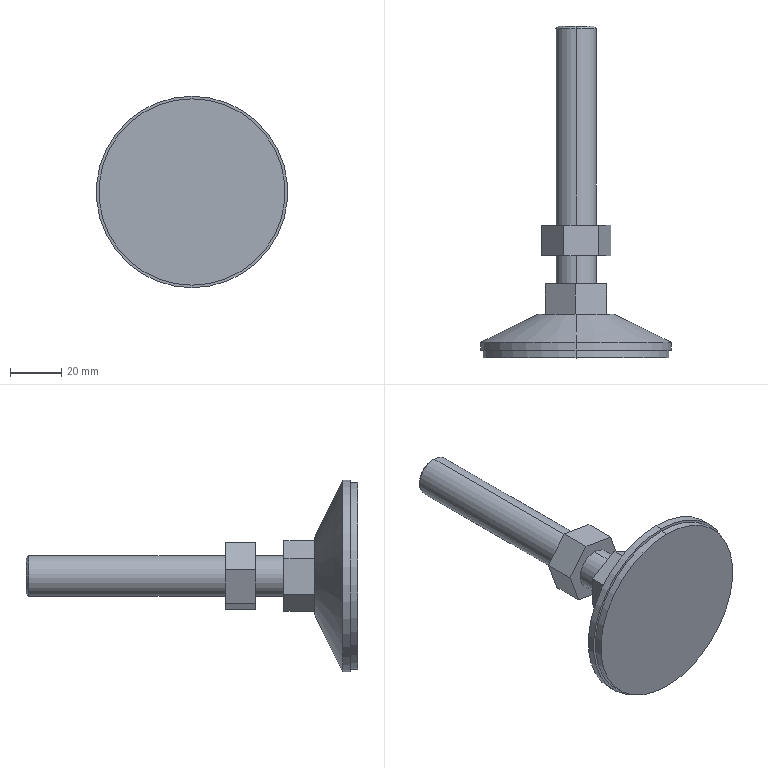Part | SolidWorks | features Boss 2, Chamfer 1, Revolution 1 | 1 solid | 31 faces | box 75 x 130 x 75 mm | volume 80922 mm3 | plane 19 | cylinder 8 | cone 4 | commonest cylinder face diameters 16 x4 73 x2 75 x2
STEP:
#1=CARTESIAN_POINT('',(0.,134.373,7.));
#2=VERTEX_POINT('',#1);
#3=CARTESIAN_POINT('',(0.,134.373,-7.));
#4=VERTEX_POINT('',#3);
#5=CARTESIAN_POINT('',(0.,134.373,0.));
#6=DIRECTION('',(0.,1.,0.));
#7=DIRECTION('',(0.,0.,1.));
#8=AXIS2_PLACEMENT_3D('',#5,#6,#7);
#9=CIRCLE('',#8,7.);
#10=EDGE_CURVE('',#2,#4,#9,.T.);
#11=ORIENTED_EDGE('',*,*,#10,.F.);
#12=CARTESIAN_POINT('',(0.,133.373,8.));
#13=VERTEX_POINT('',#12);
#14=CARTESIAN_POINT('',(0.,134.373,7.));
#15=DIRECTION('',(0.,-0.7071,0.7071));
#16=VECTOR('',#15,1000.);
#17=LINE('',#14,#16);
#18=EDGE_CURVE('',#2,#13,#17,.T.);
#19=ORIENTED_EDGE('',*,*,#18,.T.);
#20=CARTESIAN_POINT('',(0.,133.373,-8.));
#21=VERTEX_POINT('',#20);
#22=CARTESIAN_POINT('',(0.,133.373,0.));
#23=DIRECTION('',(0.,-1.,0.));
#24=DIRECTION('',(0.,0.,1.));
#25=AXIS2_PLACEMENT_3D('',#22,#23,#24);
#26=CIRCLE('',#25,8.);
#27=EDGE_CURVE('',#21,#13,#26,.T.);
#28=ORIENTED_EDGE('',*,*,#27,.F.);
#29=CARTESIAN_POINT('',(0.,134.373,-7.));
#30=DIRECTION('',(0.,-0.7071,-0.7071));
#31=VECTOR('',#30,1000.);
#32=LINE('',#29,#31);
#33=EDGE_CURVE('',#4,#21,#32,.T.);
#34=ORIENTED_EDGE('',*,*,#33,.F.);
#35=EDGE_LOOP('',(#11,#19,#28,#34));
#36=FACE_OUTER_BOUND('',#35,.T.);
#37=CARTESIAN_POINT('',(0.,134.373,0.));
#38=DIRECTION('',(0.,-1.,0.));
#39=DIRECTION('',(0.,0.,-1.));
#40=AXIS2_PLACEMENT_3D('',#37,#38,#39);
#41=CONICAL_SURFACE('',#40,7.,0.7854);
#42=ADVANCED_FACE('',(#36),#41,.T.);
#43=CARTESIAN_POINT('',(0.,56.373,-8.));
#44=VERTEX_POINT('',#43);
#45=CARTESIAN_POINT('',(0.,56.373,8.));
#46=VERTEX_POINT('',#45);
#47=CARTESIAN_POINT('',(0.,56.373,0.));
#48=DIRECTION('',(0.,-1.,0.));
#49=DIRECTION('',(0.,0.,1.));
#50=AXIS2_PLACEMENT_3D('',#47,#48,#49);
#51=CIRCLE('',#50,8.);
#52=EDGE_CURVE('',#44,#46,#51,.T.);
#53=ORIENTED_EDGE('',*,*,#52,.F.);
#54=CARTESIAN_POINT('',(0.,0.,-8.));
#55=DIRECTION('',(0.,1.,0.));
#56=VECTOR('',#55,1000.);
#57=LINE('',#54,#56);
#58=EDGE_CURVE('',#44,#21,#57,.T.);
#59=ORIENTED_EDGE('',*,*,#58,.T.);
#60=ORIENTED_EDGE('',*,*,#27,.T.);
#61=CARTESIAN_POINT('',(0.,0.,8.));
#62=DIRECTION('',(0.,1.,0.));
#63=VECTOR('',#62,1000.);
#64=LINE('',#61,#63);
#65=EDGE_CURVE('',#46,#13,#64,.T.);
#66=ORIENTED_EDGE('',*,*,#65,.F.);
#67=EDGE_LOOP('',(#53,#59,#60,#66));
#68=FACE_OUTER_BOUND('',#67,.T.);
#69=CARTESIAN_POINT('',(0.,0.,0.));
#70=DIRECTION('',(0.,1.,0.));
#71=DIRECTION('',(0.,0.,1.));
#72=AXIS2_PLACEMENT_3D('',#69,#70,#71);
#73=CYLINDRICAL_SURFACE('',#72,8.);
#74=ADVANCED_FACE('',(#68),#73,.T.);
#75=CARTESIAN_POINT('',(0.,4.373,36.5));
#76=VERTEX_POINT('',#75);
#77=CARTESIAN_POINT('',(0.,4.373,-36.5));
#78=VERTEX_POINT('',#77);
#79=CARTESIAN_POINT('',(0.,4.373,0.));
#80=DIRECTION('',(0.,1.,0.));
#81=DIRECTION('',(0.,0.,1.));
#82=AXIS2_PLACEMENT_3D('',#79,#80,#81);
#83=CIRCLE('',#82,36.5);
#84=EDGE_CURVE('',#76,#78,#83,.T.);
#85=ORIENTED_EDGE('',*,*,#84,.T.);
#86=CARTESIAN_POINT('',(0.,7.373,-36.5));
#87=VERTEX_POINT('',#86);
#88=CARTESIAN_POINT('',(0.,0.,-36.5));
#89=DIRECTION('',(0.,1.,0.));
#90=VECTOR('',#89,1000.);
#91=LINE('',#88,#90);
#92=EDGE_CURVE('',#78,#87,#91,.T.);
#93=ORIENTED_EDGE('',*,*,#92,.T.);
#94=CARTESIAN_POINT('',(0.,7.373,36.5));
#95=VERTEX_POINT('',#94);
#96=CARTESIAN_POINT('',(0.,7.373,0.));
#97=DIRECTION('',(0.,1.,0.));
#98=DIRECTION('',(0.,0.,1.));
#99=AXIS2_PLACEMENT_3D('',#96,#97,#98);
#100=CIRCLE('',#99,36.5);
#101=EDGE_CURVE('',#95,#87,#100,.T.);
#102=ORIENTED_EDGE('',*,*,#101,.F.);
#103=CARTESIAN_POINT('',(0.,0.,36.5));
#104=DIRECTION('',(0.,1.,0.));
#105=VECTOR('',#104,1000.);
#106=LINE('',#103,#105);
#107=EDGE_CURVE('',#76,#95,#106,.T.);
#108=ORIENTED_EDGE('',*,*,#107,.F.);
#109=EDGE_LOOP('',(#85,#93,#102,#108));
#110=FACE_OUTER_BOUND('',#109,.T.);
#111=CARTESIAN_POINT('',(0.,0.,0.));
#112=DIRECTION('',(0.,1.,0.));
#113=DIRECTION('',(0.,0.,1.));
#114=AXIS2_PLACEMENT_3D('',#111,#112,#113);
#115=CYLINDRICAL_SURFACE('',#114,36.5);
#116=ADVANCED_FACE('',(#110),#115,.T.);
#117=CARTESIAN_POINT('',(0.,7.373,37.5));
#118=VERTEX_POINT('',#117);
#119=CARTESIAN_POINT('',(0.,7.373,-37.5));
#120=VERTEX_POINT('',#119);
#121=CARTESIAN_POINT('',(0.,7.373,0.));
#122=DIRECTION('',(0.,1.,0.));
#123=DIRECTION('',(0.,0.,1.));
#124=AXIS2_PLACEMENT_3D('',#121,#122,#123);
#125=CIRCLE('',#124,37.5);
#126=EDGE_CURVE('',#118,#120,#125,.T.);
#127=ORIENTED_EDGE('',*,*,#126,.T.);
#128=CARTESIAN_POINT('',(0.,10.373,-37.5));
#129=VERTEX_POINT('',#128);
#130=CARTESIAN_POINT('',(0.,0.,-37.5));
#131=DIRECTION('',(0.,1.,0.));
#132=VECTOR('',#131,1000.);
#133=LINE('',#130,#132);
#134=EDGE_CURVE('',#120,#129,#133,.T.);
#135=ORIENTED_EDGE('',*,*,#134,.T.);
#136=CARTESIAN_POINT('',(0.,10.373,37.5));
#137=VERTEX_POINT('',#136);
#138=CARTESIAN_POINT('',(0.,10.373,0.));
#139=DIRECTION('',(0.,1.,0.));
#140=DIRECTION('',(0.,0.,1.));
#141=AXIS2_PLACEMENT_3D('',#138,#139,#140);
#142=CIRCLE('',#141,37.5);
#143=EDGE_CURVE('',#137,#129,#142,.T.);
#144=ORIENTED_EDGE('',*,*,#143,.F.);
#145=CARTESIAN_POINT('',(0.,0.,37.5));
#146=DIRECTION('',(0.,1.,0.));
#147=VECTOR('',#146,1000.);
#148=LINE('',#145,#147);
#149=EDGE_CURVE('',#118,#137,#148,.T.);
#150=ORIENTED_EDGE('',*,*,#149,.F.);
#151=EDGE_LOOP('',(#127,#135,#144,#150));
#152=FACE_OUTER_BOUND('',#151,.T.);
#153=CARTESIAN_POINT('',(0.,0.,0.));
#154=DIRECTION('',(0.,1.,0.));
#155=DIRECTION('',(0.,0.,1.));
#156=AXIS2_PLACEMENT_3D('',#153,#154,#155);
#157=CYLINDRICAL_SURFACE('',#156,37.5);
#158=ADVANCED_FACE('',(#152),#157,.T.);
#159=CARTESIAN_POINT('',(0.,21.373,15.));
#160=VERTEX_POINT('',#159);
#161=CARTESIAN_POINT('',(0.,21.373,-15.));
#162=VERTEX_POINT('',#161);
#163=CARTESIAN_POINT('',(0.,21.373,0.));
#164=DIRECTION('',(0.,1.,0.));
#165=DIRECTION('',(0.,0.,1.));
#166=AXIS2_PLACEMENT_3D('',#163,#164,#165);
#167=CIRCLE('',#166,15.);
#168=EDGE_CURVE('',#160,#162,#167,.T.);
#169=ORIENTED_EDGE('',*,*,#168,.F.);
#170=CARTESIAN_POINT('',(0.,21.373,15.));
#171=DIRECTION('',(0.,-0.4392,0.8984));
#172=VECTOR('',#171,1000.);
#173=LINE('',#170,#172);
#174=EDGE_CURVE('',#160,#137,#173,.T.);
#175=ORIENTED_EDGE('',*,*,#174,.T.);
#176=ORIENTED_EDGE('',*,*,#143,.T.);
#177=CARTESIAN_POINT('',(0.,21.373,-15.));
#178=DIRECTION('',(0.,-0.4392,-0.8984));
#179=VECTOR('',#178,1000.);
#180=LINE('',#177,#179);
#181=EDGE_CURVE('',#162,#129,#180,.T.);
#182=ORIENTED_EDGE('',*,*,#181,.F.);
#183=EDGE_LOOP('',(#169,#175,#176,#182));
#184=FACE_OUTER_BOUND('',#183,.T.);
#185=CARTESIAN_POINT('',(0.,21.373,0.));
#186=DIRECTION('',(0.,-1.,0.));
#187=DIRECTION('',(0.,0.,-1.));
#188=AXIS2_PLACEMENT_3D('',#185,#186,#187);
#189=CONICAL_SURFACE('',#188,15.,1.116);
#190=ADVANCED_FACE('',(#184),#189,.T.);
#191=CARTESIAN_POINT('',(0.,33.373,8.));
#192=VERTEX_POINT('',#191);
#193=CARTESIAN_POINT('',(0.,33.373,-8.));
#194=VERTEX_POINT('',#193);
#195=CARTESIAN_POINT('',(0.,33.373,0.));
#196=DIRECTION('',(0.,1.,0.));
#197=DIRECTION('',(0.,0.,-1.));
#198=AXIS2_PLACEMENT_3D('',#195,#196,#197);
#199=CIRCLE('',#198,8.);
#200=EDGE_CURVE('',#192,#194,#199,.T.);
#201=ORIENTED_EDGE('',*,*,#200,.T.);
#202=CARTESIAN_POINT('',(0.,44.373,-8.));
#203=VERTEX_POINT('',#202);
#204=CARTESIAN_POINT('',(0.,0.,-8.));
#205=DIRECTION('',(0.,1.,0.));
#206=VECTOR('',#205,1000.);
#207=LINE('',#204,#206);
#208=EDGE_CURVE('',#194,#203,#207,.T.);
#209=ORIENTED_EDGE('',*,*,#208,.T.);
#210=CARTESIAN_POINT('',(0.,44.373,8.));
#211=VERTEX_POINT('',#210);
#212=CARTESIAN_POINT('',(0.,44.373,0.));
#213=DIRECTION('',(0.,-1.,0.));
#214=DIRECTION('',(0.,0.,1.));
#215=AXIS2_PLACEMENT_3D('',#212,#213,#214);
#216=CIRCLE('',#215,8.);
#217=EDGE_CURVE('',#203,#211,#216,.T.);
#218=ORIENTED_EDGE('',*,*,#217,.T.);
#219=CARTESIAN_POINT('',(0.,0.,8.));
#220=DIRECTION('',(0.,1.,0.));
#221=VECTOR('',#220,1000.);
#222=LINE('',#219,#221);
#223=EDGE_CURVE('',#192,#211,#222,.T.);
#224=ORIENTED_EDGE('',*,*,#223,.F.);
#225=EDGE_LOOP('',(#201,#209,#218,#224));
#226=FACE_OUTER_BOUND('',#225,.T.);
#227=CARTESIAN_POINT('',(0.,0.,0.));
#228=DIRECTION('',(0.,1.,0.));
#229=DIRECTION('',(0.,0.,1.));
#230=AXIS2_PLACEMENT_3D('',#227,#228,#229);
#231=CYLINDRICAL_SURFACE('',#230,8.);
#232=ADVANCED_FACE('',(#226),#231,.T.);
#233=ORIENTED_EDGE('',*,*,#208,.F.);
#234=CARTESIAN_POINT('',(0.,33.373,0.));
#235=DIRECTION('',(0.,1.,0.));
#236=DIRECTION('',(0.,0.,-1.));
#237=AXIS2_PLACEMENT_3D('',#234,#235,#236);
#238=CIRCLE('',#237,8.);
#239=EDGE_CURVE('',#194,#192,#238,.T.);
#240=ORIENTED_EDGE('',*,*,#239,.T.);
#241=ORIENTED_EDGE('',*,*,#223,.T.);
#242=CARTESIAN_POINT('',(0.,44.373,0.));
#243=DIRECTION('',(0.,-1.,0.));
#244=DIRECTION('',(0.,0.,1.));
#245=AXIS2_PLACEMENT_3D('',#242,#243,#244);
#246=CIRCLE('',#245,8.);
#247=EDGE_CURVE('',#211,#203,#246,.T.);
#248=ORIENTED_EDGE('',*,*,#247,.T.);
#249=EDGE_LOOP('',(#233,#240,#241,#248));
#250=FACE_OUTER_BOUND('',#249,.T.);
#251=CARTESIAN_POINT('',(0.,0.,0.));
#252=DIRECTION('',(0.,1.,0.));
#253=DIRECTION('',(0.,0.,1.));
#254=AXIS2_PLACEMENT_3D('',#251,#252,#253);
#255=CYLINDRICAL_SURFACE('',#254,8.);
#256=ADVANCED_FACE('',(#250),#255,.T.);
#257=CARTESIAN_POINT('',(0.,21.373,0.));
#258=DIRECTION('',(0.,1.,0.));
#259=DIRECTION('',(0.,0.,1.));
#260=AXIS2_PLACEMENT_3D('',#257,#258,#259);
#261=CIRCLE('',#260,15.);
#262=EDGE_CURVE('',#162,#160,#261,.T.);
#263=ORIENTED_EDGE('',*,*,#262,.T.);
#264=ORIENTED_EDGE('',*,*,#168,.T.);
#265=EDGE_LOOP('',(#263,#264));
#266=FACE_OUTER_BOUND('',#265,.T.);
#267=CARTESIAN_POINT('',(11.859,21.373,7.166));
#268=VERTEX_POINT('',#267);
#269=CARTESIAN_POINT('',(12.136,21.373,-6.687));
#270=VERTEX_POINT('',#269);
#271=CARTESIAN_POINT('',(11.859,21.373,7.166));
#272=DIRECTION('',(0.01996,0.,-0.9998));
#273=VECTOR('',#272,1000.);
#274=LINE('',#271,#273);
#275=EDGE_CURVE('',#268,#270,#274,.T.);
#276=ORIENTED_EDGE('',*,*,#275,.F.);
#277=CARTESIAN_POINT('',(-0.2766,21.373,13.854));
#278=VERTEX_POINT('',#277);
#279=CARTESIAN_POINT('',(-0.2766,21.373,13.854));
#280=DIRECTION('',(0.8758,0.,-0.4826));
#281=VECTOR('',#280,1000.);
#282=LINE('',#279,#281);
#283=EDGE_CURVE('',#278,#268,#282,.T.);
#284=ORIENTED_EDGE('',*,*,#283,.F.);
#285=CARTESIAN_POINT('',(-12.136,21.373,6.687));
#286=VERTEX_POINT('',#285);
#287=CARTESIAN_POINT('',(-12.136,21.373,6.687));
#288=DIRECTION('',(0.8559,0.,0.5172));
#289=VECTOR('',#288,1000.);
#290=LINE('',#287,#289);
#291=EDGE_CURVE('',#286,#278,#290,.T.);
#292=ORIENTED_EDGE('',*,*,#291,.F.);
#293=CARTESIAN_POINT('',(-11.859,21.373,-7.166));
#294=VERTEX_POINT('',#293);
#295=CARTESIAN_POINT('',(-11.859,21.373,-7.166));
#296=DIRECTION('',(-0.01996,0.,0.9998));
#297=VECTOR('',#296,1000.);
#298=LINE('',#295,#297);
#299=EDGE_CURVE('',#294,#286,#298,.T.);
#300=ORIENTED_EDGE('',*,*,#299,.F.);
#301=CARTESIAN_POINT('',(0.2766,21.373,-13.854));
#302=VERTEX_POINT('',#301);
#303=CARTESIAN_POINT('',(0.2766,21.373,-13.854));
#304=DIRECTION('',(-0.8758,0.,0.4826));
#305=VECTOR('',#304,1000.);
#306=LINE('',#303,#305);
#307=EDGE_CURVE('',#302,#294,#306,.T.);
#308=ORIENTED_EDGE('',*,*,#307,.F.);
#309=CARTESIAN_POINT('',(12.136,21.373,-6.687));
#310=DIRECTION('',(-0.8559,0.,-0.5172));
#311=VECTOR('',#310,1000.);
#312=LINE('',#309,#311);
#313=EDGE_CURVE('',#270,#302,#312,.T.);
#314=ORIENTED_EDGE('',*,*,#313,.F.);
#315=EDGE_LOOP('',(#276,#284,#292,#300,#308,#314));
#316=FACE_BOUND('',#315,.T.);
#317=CARTESIAN_POINT('',(-15.,21.373,0.));
#318=DIRECTION('',(0.,1.,0.));
#319=DIRECTION('',(0.,0.,1.));
#320=AXIS2_PLACEMENT_3D('',#317,#318,#319);
#321=PLANE('',#320);
#322=ADVANCED_FACE('',(#266,#316),#321,.T.);
#323=ORIENTED_EDGE('',*,*,#174,.F.);
#324=ORIENTED_EDGE('',*,*,#262,.F.);
#325=ORIENTED_EDGE('',*,*,#181,.T.);
#326=CARTESIAN_POINT('',(0.,10.373,0.));
#327=DIRECTION('',(0.,1.,0.));
#328=DIRECTION('',(0.,0.,1.));
#329=AXIS2_PLACEMENT_3D('',#326,#327,#328);
#330=CIRCLE('',#329,37.5);
#331=EDGE_CURVE('',#129,#137,#330,.T.);
#332=ORIENTED_EDGE('',*,*,#331,.T.);
#333=EDGE_LOOP('',(#323,#324,#325,#332));
#334=FACE_OUTER_BOUND('',#333,.T.);
#335=CARTESIAN_POINT('',(0.,21.373,0.));
#336=DIRECTION('',(0.,-1.,0.));
#337=DIRECTION('',(0.,0.,-1.));
#338=AXIS2_PLACEMENT_3D('',#335,#336,#337);
#339=CONICAL_SURFACE('',#338,15.,1.116);
#340=ADVANCED_FACE('',(#334),#339,.T.);
#341=ORIENTED_EDGE('',*,*,#134,.F.);
#342=CARTESIAN_POINT('',(0.,7.373,0.));
#343=DIRECTION('',(0.,1.,0.));
#344=DIRECTION('',(0.,0.,1.));
#345=AXIS2_PLACEMENT_3D('',#342,#343,#344);
#346=CIRCLE('',#345,37.5);
#347=EDGE_CURVE('',#120,#118,#346,.T.);
#348=ORIENTED_EDGE('',*,*,#347,.T.);
#349=ORIENTED_EDGE('',*,*,#149,.T.);
#350=ORIENTED_EDGE('',*,*,#331,.F.);
#351=EDGE_LOOP('',(#341,#348,#349,#350));
#352=FACE_OUTER_BOUND('',#351,.T.);
#353=CARTESIAN_POINT('',(0.,0.,0.));
#354=DIRECTION('',(0.,1.,0.));
#355=DIRECTION('',(0.,0.,1.));
#356=AXIS2_PLACEMENT_3D('',#353,#354,#355);
#357=CYLINDRICAL_SURFACE('',#356,37.5);
#358=ADVANCED_FACE('',(#352),#357,.T.);
#359=ORIENTED_EDGE('',*,*,#101,.T.);
#360=CARTESIAN_POINT('',(0.,7.373,0.));
#361=DIRECTION('',(0.,1.,0.));
#362=DIRECTION('',(0.,0.,1.));
#363=AXIS2_PLACEMENT_3D('',#360,#361,#362);
#364=CIRCLE('',#363,36.5);
#365=EDGE_CURVE('',#87,#95,#364,.T.);
#366=ORIENTED_EDGE('',*,*,#365,.T.);
#367=EDGE_LOOP('',(#359,#366));
#368=FACE_BOUND('',#367,.T.);
#369=ORIENTED_EDGE('',*,*,#126,.F.);
#370=ORIENTED_EDGE('',*,*,#347,.F.);
#371=EDGE_LOOP('',(#369,#370));
#372=FACE_OUTER_BOUND('',#371,.T.);
#373=CARTESIAN_POINT('',(-37.5,7.373,0.));
#374=DIRECTION('',(0.,-1.,0.));
#375=DIRECTION('',(0.,0.,-1.));
#376=AXIS2_PLACEMENT_3D('',#373,#374,#375);
#377=PLANE('',#376);
#378=ADVANCED_FACE('',(#368,#372),#377,.T.);
#379=ORIENTED_EDGE('',*,*,#92,.F.);
#380=CARTESIAN_POINT('',(0.,4.373,0.));
#381=DIRECTION('',(0.,1.,0.));
#382=DIRECTION('',(0.,0.,1.));
#383=AXIS2_PLACEMENT_3D('',#380,#381,#382);
#384=CIRCLE('',#383,36.5);
#385=EDGE_CURVE('',#78,#76,#384,.T.);
#386=ORIENTED_EDGE('',*,*,#385,.T.);
#387=ORIENTED_EDGE('',*,*,#107,.T.);
#388=ORIENTED_EDGE('',*,*,#365,.F.);
#389=EDGE_LOOP('',(#379,#386,#387,#388));
#390=FACE_OUTER_BOUND('',#389,.T.);
#391=CARTESIAN_POINT('',(0.,0.,0.));
#392=DIRECTION('',(0.,1.,0.));
#393=DIRECTION('',(0.,0.,1.));
#394=AXIS2_PLACEMENT_3D('',#391,#392,#393);
#395=CYLINDRICAL_SURFACE('',#394,36.5);
#396=ADVANCED_FACE('',(#390),#395,.T.);
#397=ORIENTED_EDGE('',*,*,#84,.F.);
#398=ORIENTED_EDGE('',*,*,#385,.F.);
#399=EDGE_LOOP('',(#397,#398));
#400=FACE_OUTER_BOUND('',#399,.T.);
#401=CARTESIAN_POINT('',(-36.5,4.373,0.));
#402=DIRECTION('',(0.,-1.,0.));
#403=DIRECTION('',(0.,0.,-1.));
#404=AXIS2_PLACEMENT_3D('',#401,#402,#403);
#405=PLANE('',#404);
#406=ADVANCED_FACE('',(#400),#405,.T.);
#407=ORIENTED_EDGE('',*,*,#283,.T.);
#408=CARTESIAN_POINT('',(11.859,33.373,7.166));
#409=VERTEX_POINT('',#408);
#410=CARTESIAN_POINT('',(11.859,33.373,7.166));
#411=DIRECTION('',(0.,-1.,0.));
#412=VECTOR('',#411,1000.);
#413=LINE('',#410,#412);
#414=EDGE_CURVE('',#409,#268,#413,.T.);
#415=ORIENTED_EDGE('',*,*,#414,.F.);
#416=CARTESIAN_POINT('',(-0.2766,33.373,13.854));
#417=VERTEX_POINT('',#416);
#418=CARTESIAN_POINT('',(-0.2766,33.373,13.854));
#419=DIRECTION('',(0.8758,0.,-0.4826));
#420=VECTOR('',#419,1000.);
#421=LINE('',#418,#420);
#422=EDGE_CURVE('',#417,#409,#421,.T.);
#423=ORIENTED_EDGE('',*,*,#422,.F.);
#424=CARTESIAN_POINT('',(-0.2766,33.373,13.854));
#425=DIRECTION('',(0.,-1.,0.));
#426=VECTOR('',#425,1000.);
#427=LINE('',#424,#426);
#428=EDGE_CURVE('',#417,#278,#427,.T.);
#429=ORIENTED_EDGE('',*,*,#428,.T.);
#430=EDGE_LOOP('',(#407,#415,#423,#429));
#431=FACE_OUTER_BOUND('',#430,.T.);
#432=CARTESIAN_POINT('',(-0.2766,33.373,13.854));
#433=DIRECTION('',(-0.4826,0.,-0.8758));
#434=DIRECTION('',(-0.8758,0.,0.4826));
#435=AXIS2_PLACEMENT_3D('',#432,#433,#434);
#436=PLANE('',#435);
#437=ADVANCED_FACE('',(#431),#436,.F.);
#438=ORIENTED_EDGE('',*,*,#275,.T.);
#439=CARTESIAN_POINT('',(12.136,33.373,-6.687));
#440=VERTEX_POINT('',#439);
#441=CARTESIAN_POINT('',(12.136,33.373,-6.687));
#442=DIRECTION('',(0.,-1.,0.));
#443=VECTOR('',#442,1000.);
#444=LINE('',#441,#443);
#445=EDGE_CURVE('',#440,#270,#444,.T.);
#446=ORIENTED_EDGE('',*,*,#445,.F.);
#447=CARTESIAN_POINT('',(11.859,33.373,7.166));
#448=DIRECTION('',(0.01996,0.,-0.9998));
#449=VECTOR('',#448,1000.);
#450=LINE('',#447,#449);
#451=EDGE_CURVE('',#409,#440,#450,.T.);
#452=ORIENTED_EDGE('',*,*,#451,.F.);
#453=ORIENTED_EDGE('',*,*,#414,.T.);
#454=EDGE_LOOP('',(#438,#446,#452,#453));
#455=FACE_OUTER_BOUND('',#454,.T.);
#456=CARTESIAN_POINT('',(11.859,33.373,7.166));
#457=DIRECTION('',(-0.9998,0.,-0.01996));
#458=DIRECTION('',(-0.01996,0.,0.9998));
#459=AXIS2_PLACEMENT_3D('',#456,#457,#458);
#460=PLANE('',#459);
#461=ADVANCED_FACE('',(#455),#460,.F.);
#462=ORIENTED_EDGE('',*,*,#313,.T.);
#463=CARTESIAN_POINT('',(0.2766,33.373,-13.854));
#464=VERTEX_POINT('',#463);
#465=CARTESIAN_POINT('',(0.2766,33.373,-13.854));
#466=DIRECTION('',(0.,-1.,0.));
#467=VECTOR('',#466,1000.);
#468=LINE('',#465,#467);
#469=EDGE_CURVE('',#464,#302,#468,.T.);
#470=ORIENTED_EDGE('',*,*,#469,.F.);
#471=CARTESIAN_POINT('',(12.136,33.373,-6.687));
#472=DIRECTION('',(-0.8559,0.,-0.5172));
#473=VECTOR('',#472,1000.);
#474=LINE('',#471,#473);
#475=EDGE_CURVE('',#440,#464,#474,.T.);
#476=ORIENTED_EDGE('',*,*,#475,.F.);
#477=ORIENTED_EDGE('',*,*,#445,.T.);
#478=EDGE_LOOP('',(#462,#470,#476,#477));
#479=FACE_OUTER_BOUND('',#478,.T.);
#480=CARTESIAN_POINT('',(12.136,33.373,-6.687));
#481=DIRECTION('',(-0.5172,0.,0.8559));
#482=DIRECTION('',(0.8559,0.,0.5172));
#483=AXIS2_PLACEMENT_3D('',#480,#481,#482);
#484=PLANE('',#483);
#485=ADVANCED_FACE('',(#479),#484,.F.);
#486=ORIENTED_EDGE('',*,*,#307,.T.);
#487=CARTESIAN_POINT('',(-11.859,33.373,-7.166));
#488=VERTEX_POINT('',#487);
#489=CARTESIAN_POINT('',(-11.859,33.373,-7.166));
#490=DIRECTION('',(0.,-1.,0.));
#491=VECTOR('',#490,1000.);
#492=LINE('',#489,#491);
#493=EDGE_CURVE('',#488,#294,#492,.T.);
#494=ORIENTED_EDGE('',*,*,#493,.F.);
#495=CARTESIAN_POINT('',(0.2766,33.373,-13.854));
#496=DIRECTION('',(-0.8758,0.,0.4826));
#497=VECTOR('',#496,1000.);
#498=LINE('',#495,#497);
#499=EDGE_CURVE('',#464,#488,#498,.T.);
#500=ORIENTED_EDGE('',*,*,#499,.F.);
#501=ORIENTED_EDGE('',*,*,#469,.T.);
#502=EDGE_LOOP('',(#486,#494,#500,#501));
#503=FACE_OUTER_BOUND('',#502,.T.);
#504=CARTESIAN_POINT('',(0.2766,33.373,-13.854));
#505=DIRECTION('',(0.4826,0.,0.8758));
#506=DIRECTION('',(0.8758,0.,-0.4826));
#507=AXIS2_PLACEMENT_3D('',#504,#505,#506);
#508=PLANE('',#507);
#509=ADVANCED_FACE('',(#503),#508,.F.);
#510=ORIENTED_EDGE('',*,*,#299,.T.);
#511=CARTESIAN_POINT('',(-12.136,33.373,6.687));
#512=VERTEX_POINT('',#511);
#513=CARTESIAN_POINT('',(-12.136,33.373,6.687));
#514=DIRECTION('',(0.,-1.,0.));
#515=VECTOR('',#514,1000.);
#516=LINE('',#513,#515);
#517=EDGE_CURVE('',#512,#286,#516,.T.);
#518=ORIENTED_EDGE('',*,*,#517,.F.);
#519=CARTESIAN_POINT('',(-11.859,33.373,-7.166));
#520=DIRECTION('',(-0.01996,0.,0.9998));
#521=VECTOR('',#520,1000.);
#522=LINE('',#519,#521);
#523=EDGE_CURVE('',#488,#512,#522,.T.);
#524=ORIENTED_EDGE('',*,*,#523,.F.);
#525=ORIENTED_EDGE('',*,*,#493,.T.);
#526=EDGE_LOOP('',(#510,#518,#524,#525));
#527=FACE_OUTER_BOUND('',#526,.T.);
#528=CARTESIAN_POINT('',(-11.859,33.373,-7.166));
#529=DIRECTION('',(0.9998,0.,0.01996));
#530=DIRECTION('',(0.01996,0.,-0.9998));
#531=AXIS2_PLACEMENT_3D('',#528,#529,#530);
#532=PLANE('',#531);
#533=ADVANCED_FACE('',(#527),#532,.F.);
#534=ORIENTED_EDGE('',*,*,#291,.T.);
#535=ORIENTED_EDGE('',*,*,#428,.F.);
#536=CARTESIAN_POINT('',(-12.136,33.373,6.687));
#537=DIRECTION('',(0.8559,0.,0.5172));
#538=VECTOR('',#537,1000.);
#539=LINE('',#536,#538);
#540=EDGE_CURVE('',#512,#417,#539,.T.);
#541=ORIENTED_EDGE('',*,*,#540,.F.);
#542=ORIENTED_EDGE('',*,*,#517,.T.);
#543=EDGE_LOOP('',(#534,#535,#541,#542));
#544=FACE_OUTER_BOUND('',#543,.T.);
#545=CARTESIAN_POINT('',(-12.136,33.373,6.687));
#546=DIRECTION('',(0.5172,0.,-0.8559));
#547=DIRECTION('',(-0.8559,0.,-0.5172));
#548=AXIS2_PLACEMENT_3D('',#545,#546,#547);
#549=PLANE('',#548);
#550=ADVANCED_FACE('',(#544),#549,.F.);
#551=ORIENTED_EDGE('',*,*,#200,.F.);
#552=ORIENTED_EDGE('',*,*,#239,.F.);
#553=EDGE_LOOP('',(#551,#552));
#554=FACE_BOUND('',#553,.T.);
#555=ORIENTED_EDGE('',*,*,#422,.T.);
#556=ORIENTED_EDGE('',*,*,#451,.T.);
#557=ORIENTED_EDGE('',*,*,#475,.T.);
#558=ORIENTED_EDGE('',*,*,#499,.T.);
#559=ORIENTED_EDGE('',*,*,#523,.T.);
#560=ORIENTED_EDGE('',*,*,#540,.T.);
#561=EDGE_LOOP('',(#555,#556,#557,#558,#559,#560));
#562=FACE_OUTER_BOUND('',#561,.T.);
#563=CARTESIAN_POINT('',(-0.2766,33.373,13.854));
#564=DIRECTION('',(0.,-1.,0.));
#565=DIRECTION('',(0.,0.,-1.));
#566=AXIS2_PLACEMENT_3D('',#563,#564,#565);
#567=PLANE('',#566);
#568=ADVANCED_FACE('',(#554,#562),#567,.F.);
#569=CARTESIAN_POINT('',(-4.762,56.373,13.012));
#570=VERTEX_POINT('',#569);
#571=CARTESIAN_POINT('',(8.888,56.373,10.63));
#572=VERTEX_POINT('',#571);
#573=CARTESIAN_POINT('',(-4.762,56.373,13.012));
#574=DIRECTION('',(0.9851,0.,-0.1719));
#575=VECTOR('',#574,1000.);
#576=LINE('',#573,#575);
#577=EDGE_CURVE('',#570,#572,#576,.T.);
#578=ORIENTED_EDGE('',*,*,#577,.F.);
#579=CARTESIAN_POINT('',(-4.762,44.373,13.012));
#580=VERTEX_POINT('',#579);
#581=CARTESIAN_POINT('',(-4.762,44.373,13.012));
#582=DIRECTION('',(0.,1.,0.));
#583=VECTOR('',#582,1000.);
#584=LINE('',#581,#583);
#585=EDGE_CURVE('',#580,#570,#584,.T.);
#586=ORIENTED_EDGE('',*,*,#585,.F.);
#587=CARTESIAN_POINT('',(8.888,44.373,10.63));
#588=VERTEX_POINT('',#587);
#589=CARTESIAN_POINT('',(-4.762,44.373,13.012));
#590=DIRECTION('',(0.9851,0.,-0.1719));
#591=VECTOR('',#590,1000.);
#592=LINE('',#589,#591);
#593=EDGE_CURVE('',#580,#588,#592,.T.);
#594=ORIENTED_EDGE('',*,*,#593,.T.);
#595=CARTESIAN_POINT('',(8.888,44.373,10.63));
#596=DIRECTION('',(0.,1.,0.));
#597=VECTOR('',#596,1000.);
#598=LINE('',#595,#597);
#599=EDGE_CURVE('',#588,#572,#598,.T.);
#600=ORIENTED_EDGE('',*,*,#599,.T.);
#601=EDGE_LOOP('',(#578,#586,#594,#600));
#602=FACE_OUTER_BOUND('',#601,.T.);
#603=CARTESIAN_POINT('',(-4.762,44.373,13.012));
#604=DIRECTION('',(0.1719,0.,0.9851));
#605=DIRECTION('',(0.9851,0.,-0.1719));
#606=AXIS2_PLACEMENT_3D('',#603,#604,#605);
#607=PLANE('',#606);
#608=ADVANCED_FACE('',(#602),#607,.T.);
#609=CARTESIAN_POINT('',(-13.65,56.373,2.382));
#610=VERTEX_POINT('',#609);
#611=CARTESIAN_POINT('',(-13.65,56.373,2.382));
#612=DIRECTION('',(0.6414,0.,0.7672));
#613=VECTOR('',#612,1000.);
#614=LINE('',#611,#613);
#615=EDGE_CURVE('',#610,#570,#614,.T.);
#616=ORIENTED_EDGE('',*,*,#615,.F.);
#617=CARTESIAN_POINT('',(-13.65,44.373,2.382));
#618=VERTEX_POINT('',#617);
#619=CARTESIAN_POINT('',(-13.65,44.373,2.382));
#620=DIRECTION('',(0.,1.,0.));
#621=VECTOR('',#620,1000.);
#622=LINE('',#619,#621);
#623=EDGE_CURVE('',#618,#610,#622,.T.);
#624=ORIENTED_EDGE('',*,*,#623,.F.);
#625=CARTESIAN_POINT('',(-13.65,44.373,2.382));
#626=DIRECTION('',(0.6414,0.,0.7672));
#627=VECTOR('',#626,1000.);
#628=LINE('',#625,#627);
#629=EDGE_CURVE('',#618,#580,#628,.T.);
#630=ORIENTED_EDGE('',*,*,#629,.T.);
#631=ORIENTED_EDGE('',*,*,#585,.T.);
#632=EDGE_LOOP('',(#616,#624,#630,#631));
#633=FACE_OUTER_BOUND('',#632,.T.);
#634=CARTESIAN_POINT('',(-13.65,44.373,2.382));
#635=DIRECTION('',(-0.7672,0.,0.6414));
#636=DIRECTION('',(0.6414,0.,0.7672));
#637=AXIS2_PLACEMENT_3D('',#634,#635,#636);
#638=PLANE('',#637);
#639=ADVANCED_FACE('',(#633),#638,.T.);
#640=CARTESIAN_POINT('',(-8.888,56.373,-10.63));
#641=VERTEX_POINT('',#640);
#642=CARTESIAN_POINT('',(-8.888,56.373,-10.63));
#643=DIRECTION('',(-0.3437,0.,0.9391));
#644=VECTOR('',#643,1000.);
#645=LINE('',#642,#644);
#646=EDGE_CURVE('',#641,#610,#645,.T.);
#647=ORIENTED_EDGE('',*,*,#646,.F.);
#648=CARTESIAN_POINT('',(-8.888,44.373,-10.63));
#649=VERTEX_POINT('',#648);
#650=CARTESIAN_POINT('',(-8.888,44.373,-10.63));
#651=DIRECTION('',(0.,1.,0.));
#652=VECTOR('',#651,1000.);
#653=LINE('',#650,#652);
#654=EDGE_CURVE('',#649,#641,#653,.T.);
#655=ORIENTED_EDGE('',*,*,#654,.F.);
#656=CARTESIAN_POINT('',(-8.888,44.373,-10.63));
#657=DIRECTION('',(-0.3437,0.,0.9391));
#658=VECTOR('',#657,1000.);
#659=LINE('',#656,#658);
#660=EDGE_CURVE('',#649,#618,#659,.T.);
#661=ORIENTED_EDGE('',*,*,#660,.T.);
#662=ORIENTED_EDGE('',*,*,#623,.T.);
#663=EDGE_LOOP('',(#647,#655,#661,#662));
#664=FACE_OUTER_BOUND('',#663,.T.);
#665=CARTESIAN_POINT('',(-8.888,44.373,-10.63));
#666=DIRECTION('',(-0.9391,0.,-0.3437));
#667=DIRECTION('',(-0.3437,0.,0.9391));
#668=AXIS2_PLACEMENT_3D('',#665,#666,#667);
#669=PLANE('',#668);
#670=ADVANCED_FACE('',(#664),#669,.T.);
#671=CARTESIAN_POINT('',(4.762,56.373,-13.012));
#672=VERTEX_POINT('',#671);
#673=CARTESIAN_POINT('',(4.762,56.373,-13.012));
#674=DIRECTION('',(-0.9851,0.,0.1719));
#675=VECTOR('',#674,1000.);
#676=LINE('',#673,#675);
#677=EDGE_CURVE('',#672,#641,#676,.T.);
#678=ORIENTED_EDGE('',*,*,#677,.F.);
#679=CARTESIAN_POINT('',(4.762,44.373,-13.012));
#680=VERTEX_POINT('',#679);
#681=CARTESIAN_POINT('',(4.762,44.373,-13.012));
#682=DIRECTION('',(0.,1.,0.));
#683=VECTOR('',#682,1000.);
#684=LINE('',#681,#683);
#685=EDGE_CURVE('',#680,#672,#684,.T.);
#686=ORIENTED_EDGE('',*,*,#685,.F.);
#687=CARTESIAN_POINT('',(4.762,44.373,-13.012));
#688=DIRECTION('',(-0.9851,0.,0.1719));
#689=VECTOR('',#688,1000.);
#690=LINE('',#687,#689);
#691=EDGE_CURVE('',#680,#649,#690,.T.);
#692=ORIENTED_EDGE('',*,*,#691,.T.);
#693=ORIENTED_EDGE('',*,*,#654,.T.);
#694=EDGE_LOOP('',(#678,#686,#692,#693));
#695=FACE_OUTER_BOUND('',#694,.T.);
#696=CARTESIAN_POINT('',(4.762,44.373,-13.012));
#697=DIRECTION('',(-0.1719,0.,-0.9851));
#698=DIRECTION('',(-0.9851,0.,0.1719));
#699=AXIS2_PLACEMENT_3D('',#696,#697,#698);
#700=PLANE('',#699);
#701=ADVANCED_FACE('',(#695),#700,.T.);
#702=CARTESIAN_POINT('',(13.65,56.373,-2.382));
#703=VERTEX_POINT('',#702);
#704=CARTESIAN_POINT('',(13.65,56.373,-2.382));
#705=DIRECTION('',(-0.6414,0.,-0.7672));
#706=VECTOR('',#705,1000.);
#707=LINE('',#704,#706);
#708=EDGE_CURVE('',#703,#672,#707,.T.);
#709=ORIENTED_EDGE('',*,*,#708,.F.);
#710=CARTESIAN_POINT('',(13.65,44.373,-2.382));
#711=VERTEX_POINT('',#710);
#712=CARTESIAN_POINT('',(13.65,44.373,-2.382));
#713=DIRECTION('',(0.,1.,0.));
#714=VECTOR('',#713,1000.);
#715=LINE('',#712,#714);
#716=EDGE_CURVE('',#711,#703,#715,.T.);
#717=ORIENTED_EDGE('',*,*,#716,.F.);
#718=CARTESIAN_POINT('',(13.65,44.373,-2.382));
#719=DIRECTION('',(-0.6414,0.,-0.7672));
#720=VECTOR('',#719,1000.);
#721=LINE('',#718,#720);
#722=EDGE_CURVE('',#711,#680,#721,.T.);
#723=ORIENTED_EDGE('',*,*,#722,.T.);
#724=ORIENTED_EDGE('',*,*,#685,.T.);
#725=EDGE_LOOP('',(#709,#717,#723,#724));
#726=FACE_OUTER_BOUND('',#725,.T.);
#727=CARTESIAN_POINT('',(13.65,44.373,-2.382));
#728=DIRECTION('',(0.7672,0.,-0.6414));
#729=DIRECTION('',(-0.6414,0.,-0.7672));
#730=AXIS2_PLACEMENT_3D('',#727,#728,#729);
#731=PLANE('',#730);
#732=ADVANCED_FACE('',(#726),#731,.T.);
#733=CARTESIAN_POINT('',(8.888,56.373,10.63));
#734=DIRECTION('',(0.3437,0.,-0.9391));
#735=VECTOR('',#734,1000.);
#736=LINE('',#733,#735);
#737=EDGE_CURVE('',#572,#703,#736,.T.);
#738=ORIENTED_EDGE('',*,*,#737,.F.);
#739=ORIENTED_EDGE('',*,*,#599,.F.);
#740=CARTESIAN_POINT('',(8.888,44.373,10.63));
#741=DIRECTION('',(0.3437,0.,-0.9391));
#742=VECTOR('',#741,1000.);
#743=LINE('',#740,#742);
#744=EDGE_CURVE('',#588,#711,#743,.T.);
#745=ORIENTED_EDGE('',*,*,#744,.T.);
#746=ORIENTED_EDGE('',*,*,#716,.T.);
#747=EDGE_LOOP('',(#738,#739,#745,#746));
#748=FACE_OUTER_BOUND('',#747,.T.);
#749=CARTESIAN_POINT('',(8.888,44.373,10.63));
#750=DIRECTION('',(0.9391,0.,0.3437));
#751=DIRECTION('',(0.3437,0.,-0.9391));
#752=AXIS2_PLACEMENT_3D('',#749,#750,#751);
#753=PLANE('',#752);
#754=ADVANCED_FACE('',(#748),#753,.T.);
#755=ORIENTED_EDGE('',*,*,#247,.F.);
#756=ORIENTED_EDGE('',*,*,#217,.F.);
#757=EDGE_LOOP('',(#755,#756));
#758=FACE_BOUND('',#757,.T.);
#759=ORIENTED_EDGE('',*,*,#593,.F.);
#760=ORIENTED_EDGE('',*,*,#629,.F.);
#761=ORIENTED_EDGE('',*,*,#660,.F.);
#762=ORIENTED_EDGE('',*,*,#691,.F.);
#763=ORIENTED_EDGE('',*,*,#722,.F.);
#764=ORIENTED_EDGE('',*,*,#744,.F.);
#765=EDGE_LOOP('',(#759,#760,#761,#762,#763,#764));
#766=FACE_OUTER_BOUND('',#765,.T.);
#767=CARTESIAN_POINT('',(8.888,44.373,10.63));
#768=DIRECTION('',(0.,1.,0.));
#769=DIRECTION('',(0.,0.,1.));
#770=AXIS2_PLACEMENT_3D('',#767,#768,#769);
#771=PLANE('',#770);
#772=ADVANCED_FACE('',(#758,#766),#771,.F.);
#773=CARTESIAN_POINT('',(0.,56.373,0.));
#774=DIRECTION('',(0.,-1.,0.));
#775=DIRECTION('',(0.,0.,1.));
#776=AXIS2_PLACEMENT_3D('',#773,#774,#775);
#777=CIRCLE('',#776,8.);
#778=EDGE_CURVE('',#46,#44,#777,.T.);
#779=ORIENTED_EDGE('',*,*,#778,.T.);
#780=ORIENTED_EDGE('',*,*,#52,.T.);
#781=EDGE_LOOP('',(#779,#780));
#782=FACE_BOUND('',#781,.T.);
#783=ORIENTED_EDGE('',*,*,#577,.T.);
#784=ORIENTED_EDGE('',*,*,#737,.T.);
#785=ORIENTED_EDGE('',*,*,#708,.T.);
#786=ORIENTED_EDGE('',*,*,#677,.T.);
#787=ORIENTED_EDGE('',*,*,#646,.T.);
#788=ORIENTED_EDGE('',*,*,#615,.T.);
#789=EDGE_LOOP('',(#783,#784,#785,#786,#787,#788));
#790=FACE_OUTER_BOUND('',#789,.T.);
#791=CARTESIAN_POINT('',(8.888,56.373,10.63));
#792=DIRECTION('',(0.,1.,0.));
#793=DIRECTION('',(0.,0.,1.));
#794=AXIS2_PLACEMENT_3D('',#791,#792,#793);
#795=PLANE('',#794);
#796=ADVANCED_FACE('',(#782,#790),#795,.T.);
#797=CARTESIAN_POINT('',(0.,134.373,0.));
#798=DIRECTION('',(0.,1.,0.));
#799=DIRECTION('',(0.,0.,1.));
#800=AXIS2_PLACEMENT_3D('',#797,#798,#799);
#801=CIRCLE('',#800,7.);
#802=EDGE_CURVE('',#4,#2,#801,.T.);
#803=ORIENTED_EDGE('',*,*,#802,.T.);
#804=ORIENTED_EDGE('',*,*,#10,.T.);
#805=EDGE_LOOP('',(#803,#804));
#806=FACE_OUTER_BOUND('',#805,.T.);
#807=CARTESIAN_POINT('',(0.,134.373,0.));
#808=DIRECTION('',(0.,1.,0.));
#809=DIRECTION('',(0.,0.,1.));
#810=AXIS2_PLACEMENT_3D('',#807,#808,#809);
#811=PLANE('',#810);
#812=ADVANCED_FACE('',(#806),#811,.T.);
#813=ORIENTED_EDGE('',*,*,#58,.F.);
#814=ORIENTED_EDGE('',*,*,#778,.F.);
#815=ORIENTED_EDGE('',*,*,#65,.T.);
#816=CARTESIAN_POINT('',(0.,133.373,0.));
#817=DIRECTION('',(0.,-1.,0.));
#818=DIRECTION('',(0.,0.,1.));
#819=AXIS2_PLACEMENT_3D('',#816,#817,#818);
#820=CIRCLE('',#819,8.);
#821=EDGE_CURVE('',#13,#21,#820,.T.);
#822=ORIENTED_EDGE('',*,*,#821,.T.);
#823=EDGE_LOOP('',(#813,#814,#815,#822));
#824=FACE_OUTER_BOUND('',#823,.T.);
#825=CARTESIAN_POINT('',(0.,0.,0.));
#826=DIRECTION('',(0.,1.,0.));
#827=DIRECTION('',(0.,0.,1.));
#828=AXIS2_PLACEMENT_3D('',#825,#826,#827);
#829=CYLINDRICAL_SURFACE('',#828,8.);
#830=ADVANCED_FACE('',(#824),#829,.T.);
#831=ORIENTED_EDGE('',*,*,#18,.F.);
#832=ORIENTED_EDGE('',*,*,#802,.F.);
#833=ORIENTED_EDGE('',*,*,#33,.T.);
#834=ORIENTED_EDGE('',*,*,#821,.F.);
#835=EDGE_LOOP('',(#831,#832,#833,#834));
#836=FACE_OUTER_BOUND('',#835,.T.);
#837=CARTESIAN_POINT('',(0.,134.373,0.));
#838=DIRECTION('',(0.,-1.,0.));
#839=DIRECTION('',(0.,0.,-1.));
#840=AXIS2_PLACEMENT_3D('',#837,#838,#839);
#841=CONICAL_SURFACE('',#840,7.,0.7854);
#842=ADVANCED_FACE('',(#836),#841,.T.);
#843=CLOSED_SHELL('',(#42,#74,#116,#158,#190,#232,#256,#322,#340,#358,#378,#396,#406,#437,#461,#485,#509,#533,#550,#568,#608,#639,#670,#701,#732,#754,#772,#796,#812,#830,#842));
#844=MANIFOLD_SOLID_BREP('',#843);
#845=CARTESIAN_POINT('',(0.,0.,0.));
#846=DIRECTION('',(0.,0.,1.));
#847=DIRECTION('',(1.,0.,0.));
#848=AXIS2_PLACEMENT_3D('',#845,#846,#847);
#849=(LENGTH_UNIT()NAMED_UNIT(*)SI_UNIT(.MILLI.,.METRE.));
#850=UNCERTAINTY_MEASURE_WITH_UNIT(LENGTH_MEASURE(0.00001),#849,'','');
#851=(NAMED_UNIT(*)PLANE_ANGLE_UNIT()SI_UNIT($,.RADIAN.));
#852=(NAMED_UNIT(*)SI_UNIT($,.STERADIAN.)SOLID_ANGLE_UNIT());
#853=(GEOMETRIC_REPRESENTATION_CONTEXT(3)GLOBAL_UNCERTAINTY_ASSIGNED_CONTEXT((#850))GLOBAL_UNIT_ASSIGNED_CONTEXT((#849,#851,#852))REPRESENTATION_CONTEXT('',''));
#854=ADVANCED_BREP_SHAPE_REPRESENTATION('',(#844,#848),#853);